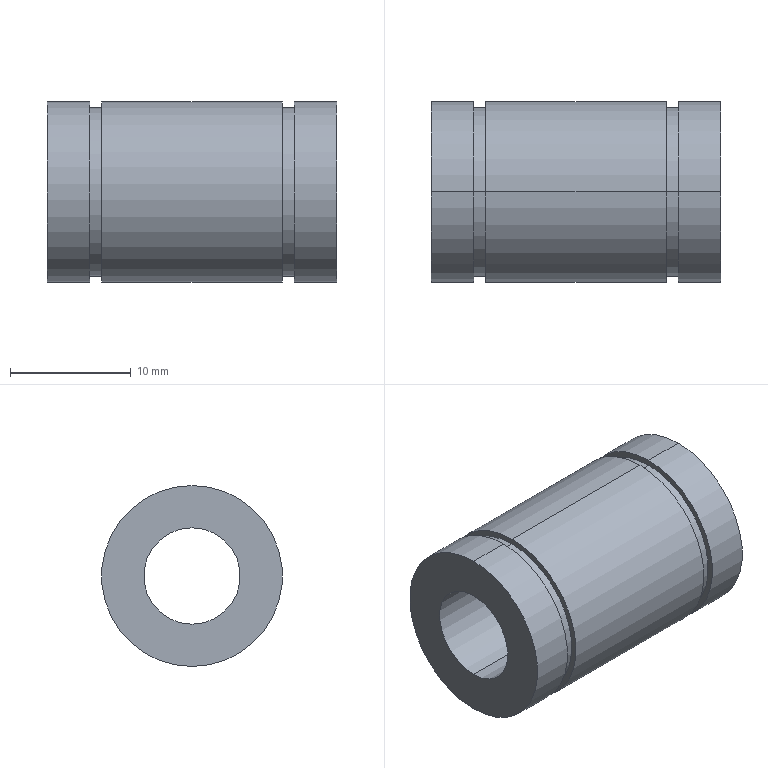Part | STEP file | linear bearing LM8-8-15-24 | 1 solid | 18 faces | box 24 x 15 x 15 mm | volume 2989 mm3 | cylinder 12 | plane 6 | commonest cylinder face diameters 15 x6 14 x4 8 x2
STEP:
#1=CARTESIAN_POINT('',(0.,0.,0.));
#2=DIRECTION('',(0.,0.,1.));
#3=DIRECTION('',(1.,0.,0.));
#4=AXIS2_PLACEMENT_3D('',#1,#2,#3);
#5=CARTESIAN_POINT('',(-20.214,0.,4.));
#6=VERTEX_POINT('',#5);
#7=CARTESIAN_POINT('',(-44.214,0.,4.));
#8=VERTEX_POINT('',#7);
#9=CARTESIAN_POINT('',(-96.213,0.,4.));
#10=DIRECTION('',(-1.,0.,0.));
#11=VECTOR('',#10,1.);
#12=LINE('',#9,#11);
#13=CARTESIAN_POINT('',(-96.213,0.,0.));
#14=DIRECTION('',(-1.,0.,0.));
#15=DIRECTION('',(0.,0.,1.));
#16=AXIS2_PLACEMENT_3D('',#13,#14,#15);
#17=CYLINDRICAL_SURFACE('',#16,4.);
#18=CARTESIAN_POINT('',(6.283,0.));
#19=DIRECTION('',(0.,1.));
#20=VECTOR('',#19,1.);
#21=LINE('',#18,#20);
#22=(GEOMETRIC_REPRESENTATION_CONTEXT(2)PARAMETRIC_REPRESENTATION_CONTEXT()REPRESENTATION_CONTEXT('',''));
#23=DEFINITIONAL_REPRESENTATION('',(#21),#22);
#24=PCURVE('',#17,#23);
#25=CARTESIAN_POINT('',(-96.213,0.,0.));
#26=DIRECTION('',(-1.,0.,0.));
#27=DIRECTION('',(0.,0.,1.));
#28=AXIS2_PLACEMENT_3D('',#25,#26,#27);
#29=CYLINDRICAL_SURFACE('',#28,4.);
#30=CARTESIAN_POINT('',(0.,0.));
#31=DIRECTION('',(0.,1.));
#32=VECTOR('',#31,1.);
#33=LINE('',#30,#32);
#34=(GEOMETRIC_REPRESENTATION_CONTEXT(2)PARAMETRIC_REPRESENTATION_CONTEXT()REPRESENTATION_CONTEXT('',''));
#35=DEFINITIONAL_REPRESENTATION('',(#33),#34);
#36=PCURVE('',#29,#35);
#37=SURFACE_CURVE('',#12,(#24,#36),.PCURVE_S1.);
#38=EDGE_CURVE('',#6,#8,#37,.T.);
#39=ORIENTED_EDGE('',*,*,#38,.T.);
#40=CARTESIAN_POINT('',(-44.214,0.,-4.));
#41=VERTEX_POINT('',#40);
#42=CARTESIAN_POINT('',(-44.214,0.,0.));
#43=DIRECTION('',(-1.,0.,0.));
#44=DIRECTION('',(0.,0.,1.));
#45=AXIS2_PLACEMENT_3D('',#42,#43,#44);
#46=CIRCLE('',#45,4.);
#47=CARTESIAN_POINT('',(0.,-51.999));
#48=DIRECTION('',(1.,0.));
#49=VECTOR('',#48,1.);
#50=LINE('',#47,#49);
#51=(GEOMETRIC_REPRESENTATION_CONTEXT(2)PARAMETRIC_REPRESENTATION_CONTEXT()REPRESENTATION_CONTEXT('',''));
#52=DEFINITIONAL_REPRESENTATION('',(#50),#51);
#53=PCURVE('',#17,#52);
#54=CARTESIAN_POINT('',(-44.214,4.,0.));
#55=DIRECTION('',(1.,0.,0.));
#56=DIRECTION('',(0.,0.,-1.));
#57=AXIS2_PLACEMENT_3D('',#54,#55,#56);
#58=PLANE('',#57);
#59=CARTESIAN_POINT('',(-4.,-4.));
#60=CARTESIAN_POINT('',(-4.,2.928));
#61=CARTESIAN_POINT('',(2.,-0.5359));
#62=CARTESIAN_POINT('',(8.,-4.));
#63=CARTESIAN_POINT('',(2.,-7.464));
#64=CARTESIAN_POINT('',(-4.,-10.928));
#65=CARTESIAN_POINT('',(-4.,-4.));
#66=(BOUNDED_CURVE()B_SPLINE_CURVE(2,(#59,#60,#61,#62,#63,#64,#65),.UNSPECIFIED.,.T.,.F.)B_SPLINE_CURVE_WITH_KNOTS((1,2,2,2,2,1),(-2.094,0.,2.094,4.189,6.283,8.378),.UNSPECIFIED.)CURVE()GEOMETRIC_REPRESENTATION_ITEM()RATIONAL_B_SPLINE_CURVE((1.,0.5,1.,0.5,1.,0.5,1.))REPRESENTATION_ITEM(''));
#67=(GEOMETRIC_REPRESENTATION_CONTEXT(2)PARAMETRIC_REPRESENTATION_CONTEXT()REPRESENTATION_CONTEXT('',''));
#68=DEFINITIONAL_REPRESENTATION('',(#66),#67);
#69=PCURVE('',#58,#68);
#70=SURFACE_CURVE('',#46,(#53,#69),.PCURVE_S1.);
#71=EDGE_CURVE('',#41,#8,#70,.T.);
#72=ORIENTED_EDGE('',*,*,#71,.F.);
#73=CARTESIAN_POINT('',(-20.214,0.,-4.));
#74=VERTEX_POINT('',#73);
#75=CARTESIAN_POINT('',(-96.213,0.,-4.));
#76=DIRECTION('',(-1.,0.,0.));
#77=VECTOR('',#76,1.);
#78=LINE('',#75,#77);
#79=CARTESIAN_POINT('',(3.142,0.));
#80=DIRECTION('',(0.,1.));
#81=VECTOR('',#80,1.);
#82=LINE('',#79,#81);
#83=(GEOMETRIC_REPRESENTATION_CONTEXT(2)PARAMETRIC_REPRESENTATION_CONTEXT()REPRESENTATION_CONTEXT('',''));
#84=DEFINITIONAL_REPRESENTATION('',(#82),#83);
#85=PCURVE('',#17,#84);
#86=CARTESIAN_POINT('',(3.142,0.));
#87=DIRECTION('',(0.,1.));
#88=VECTOR('',#87,1.);
#89=LINE('',#86,#88);
#90=(GEOMETRIC_REPRESENTATION_CONTEXT(2)PARAMETRIC_REPRESENTATION_CONTEXT()REPRESENTATION_CONTEXT('',''));
#91=DEFINITIONAL_REPRESENTATION('',(#89),#90);
#92=PCURVE('',#29,#91);
#93=SURFACE_CURVE('',#78,(#85,#92),.PCURVE_S1.);
#94=EDGE_CURVE('',#74,#41,#93,.T.);
#95=ORIENTED_EDGE('',*,*,#94,.F.);
#96=CARTESIAN_POINT('',(-20.214,0.,0.));
#97=DIRECTION('',(-1.,0.,0.));
#98=DIRECTION('',(0.,0.,1.));
#99=AXIS2_PLACEMENT_3D('',#96,#97,#98);
#100=CIRCLE('',#99,4.);
#101=CARTESIAN_POINT('',(0.,-75.999));
#102=DIRECTION('',(1.,0.));
#103=VECTOR('',#102,1.);
#104=LINE('',#101,#103);
#105=(GEOMETRIC_REPRESENTATION_CONTEXT(2)PARAMETRIC_REPRESENTATION_CONTEXT()REPRESENTATION_CONTEXT('',''));
#106=DEFINITIONAL_REPRESENTATION('',(#104),#105);
#107=PCURVE('',#17,#106);
#108=CARTESIAN_POINT('',(-20.214,4.,0.));
#109=DIRECTION('',(-1.,0.,0.));
#110=DIRECTION('',(0.,0.,1.));
#111=AXIS2_PLACEMENT_3D('',#108,#109,#110);
#112=PLANE('',#111);
#113=CARTESIAN_POINT('',(0.,-4.));
#114=DIRECTION('',(1.,0.));
#115=AXIS2_PLACEMENT_2D('',#113,#114);
#116=CIRCLE('',#115,4.);
#117=(GEOMETRIC_REPRESENTATION_CONTEXT(2)PARAMETRIC_REPRESENTATION_CONTEXT()REPRESENTATION_CONTEXT('',''));
#118=DEFINITIONAL_REPRESENTATION('',(#116),#117);
#119=PCURVE('',#112,#118);
#120=SURFACE_CURVE('',#100,(#107,#119),.PCURVE_S1.);
#121=EDGE_CURVE('',#74,#6,#120,.T.);
#122=ORIENTED_EDGE('',*,*,#121,.T.);
#123=EDGE_LOOP('',(#39,#72,#95,#122));
#124=FACE_BOUND('',#123,.F.);
#125=ADVANCED_FACE('',(#124),#17,.F.);
#126=CARTESIAN_POINT('',(-20.214,0.,7.5));
#127=VERTEX_POINT('',#126);
#128=CARTESIAN_POINT('',(-20.214,0.,-7.5));
#129=VERTEX_POINT('',#128);
#130=CARTESIAN_POINT('',(-20.214,0.,0.));
#131=DIRECTION('',(-1.,0.,0.));
#132=DIRECTION('',(0.,0.,1.));
#133=AXIS2_PLACEMENT_3D('',#130,#131,#132);
#134=CIRCLE('',#133,7.5);
#135=CARTESIAN_POINT('',(-96.213,0.,0.));
#136=DIRECTION('',(-1.,0.,0.));
#137=DIRECTION('',(0.,0.,1.));
#138=AXIS2_PLACEMENT_3D('',#135,#136,#137);
#139=CYLINDRICAL_SURFACE('',#138,7.5);
#140=CARTESIAN_POINT('',(0.,-75.999));
#141=DIRECTION('',(1.,0.));
#142=VECTOR('',#141,1.);
#143=LINE('',#140,#142);
#144=(GEOMETRIC_REPRESENTATION_CONTEXT(2)PARAMETRIC_REPRESENTATION_CONTEXT()REPRESENTATION_CONTEXT('',''));
#145=DEFINITIONAL_REPRESENTATION('',(#143),#144);
#146=PCURVE('',#139,#145);
#147=CARTESIAN_POINT('',(0.,-4.));
#148=DIRECTION('',(1.,0.));
#149=AXIS2_PLACEMENT_2D('',#147,#148);
#150=CIRCLE('',#149,7.5);
#151=(GEOMETRIC_REPRESENTATION_CONTEXT(2)PARAMETRIC_REPRESENTATION_CONTEXT()REPRESENTATION_CONTEXT('',''));
#152=DEFINITIONAL_REPRESENTATION('',(#150),#151);
#153=PCURVE('',#112,#152);
#154=SURFACE_CURVE('',#134,(#146,#153),.PCURVE_S1.);
#155=EDGE_CURVE('',#127,#129,#154,.T.);
#156=ORIENTED_EDGE('',*,*,#155,.T.);
#157=CARTESIAN_POINT('',(-23.714,0.,-7.5));
#158=VERTEX_POINT('',#157);
#159=CARTESIAN_POINT('',(-96.213,0.,-7.5));
#160=DIRECTION('',(-1.,0.,0.));
#161=VECTOR('',#160,1.);
#162=LINE('',#159,#161);
#163=CARTESIAN_POINT('',(3.142,0.));
#164=DIRECTION('',(0.,1.));
#165=VECTOR('',#164,1.);
#166=LINE('',#163,#165);
#167=(GEOMETRIC_REPRESENTATION_CONTEXT(2)PARAMETRIC_REPRESENTATION_CONTEXT()REPRESENTATION_CONTEXT('',''));
#168=DEFINITIONAL_REPRESENTATION('',(#166),#167);
#169=PCURVE('',#139,#168);
#170=CARTESIAN_POINT('',(-96.213,0.,0.));
#171=DIRECTION('',(-1.,0.,0.));
#172=DIRECTION('',(0.,0.,1.));
#173=AXIS2_PLACEMENT_3D('',#170,#171,#172);
#174=CYLINDRICAL_SURFACE('',#173,7.5);
#175=CARTESIAN_POINT('',(3.142,0.));
#176=DIRECTION('',(0.,1.));
#177=VECTOR('',#176,1.);
#178=LINE('',#175,#177);
#179=(GEOMETRIC_REPRESENTATION_CONTEXT(2)PARAMETRIC_REPRESENTATION_CONTEXT()REPRESENTATION_CONTEXT('',''));
#180=DEFINITIONAL_REPRESENTATION('',(#178),#179);
#181=PCURVE('',#174,#180);
#182=SURFACE_CURVE('',#162,(#169,#181),.PCURVE_S1.);
#183=EDGE_CURVE('',#129,#158,#182,.T.);
#184=ORIENTED_EDGE('',*,*,#183,.T.);
#185=CARTESIAN_POINT('',(-23.714,0.,7.5));
#186=VERTEX_POINT('',#185);
#187=CARTESIAN_POINT('',(-23.714,0.,0.));
#188=DIRECTION('',(-1.,0.,0.));
#189=DIRECTION('',(0.,0.,1.));
#190=AXIS2_PLACEMENT_3D('',#187,#188,#189);
#191=CIRCLE('',#190,7.5);
#192=CARTESIAN_POINT('',(0.,-72.499));
#193=DIRECTION('',(1.,0.));
#194=VECTOR('',#193,1.);
#195=LINE('',#192,#194);
#196=(GEOMETRIC_REPRESENTATION_CONTEXT(2)PARAMETRIC_REPRESENTATION_CONTEXT()REPRESENTATION_CONTEXT('',''));
#197=DEFINITIONAL_REPRESENTATION('',(#195),#196);
#198=PCURVE('',#139,#197);
#199=CARTESIAN_POINT('',(-23.714,7.5,0.));
#200=DIRECTION('',(1.,0.,0.));
#201=DIRECTION('',(0.,0.,-1.));
#202=AXIS2_PLACEMENT_3D('',#199,#200,#201);
#203=PLANE('',#202);
#204=CARTESIAN_POINT('',(-7.5,-7.5));
#205=CARTESIAN_POINT('',(-7.5,5.49));
#206=CARTESIAN_POINT('',(3.75,-1.005));
#207=CARTESIAN_POINT('',(15.,-7.5));
#208=CARTESIAN_POINT('',(3.75,-13.995));
#209=CARTESIAN_POINT('',(-7.5,-20.49));
#210=CARTESIAN_POINT('',(-7.5,-7.5));
#211=(BOUNDED_CURVE()B_SPLINE_CURVE(2,(#204,#205,#206,#207,#208,#209,#210),.UNSPECIFIED.,.T.,.F.)B_SPLINE_CURVE_WITH_KNOTS((1,2,2,2,2,1),(-2.094,0.,2.094,4.189,6.283,8.378),.UNSPECIFIED.)CURVE()GEOMETRIC_REPRESENTATION_ITEM()RATIONAL_B_SPLINE_CURVE((1.,0.5,1.,0.5,1.,0.5,1.))REPRESENTATION_ITEM(''));
#212=(GEOMETRIC_REPRESENTATION_CONTEXT(2)PARAMETRIC_REPRESENTATION_CONTEXT()REPRESENTATION_CONTEXT('',''));
#213=DEFINITIONAL_REPRESENTATION('',(#211),#212);
#214=PCURVE('',#203,#213);
#215=SURFACE_CURVE('',#191,(#198,#214),.PCURVE_S1.);
#216=EDGE_CURVE('',#186,#158,#215,.T.);
#217=ORIENTED_EDGE('',*,*,#216,.F.);
#218=CARTESIAN_POINT('',(-96.213,0.,7.5));
#219=DIRECTION('',(-1.,0.,0.));
#220=VECTOR('',#219,1.);
#221=LINE('',#218,#220);
#222=CARTESIAN_POINT('',(0.,0.));
#223=DIRECTION('',(0.,1.));
#224=VECTOR('',#223,1.);
#225=LINE('',#222,#224);
#226=(GEOMETRIC_REPRESENTATION_CONTEXT(2)PARAMETRIC_REPRESENTATION_CONTEXT()REPRESENTATION_CONTEXT('',''));
#227=DEFINITIONAL_REPRESENTATION('',(#225),#226);
#228=PCURVE('',#139,#227);
#229=CARTESIAN_POINT('',(6.283,0.));
#230=DIRECTION('',(0.,1.));
#231=VECTOR('',#230,1.);
#232=LINE('',#229,#231);
#233=(GEOMETRIC_REPRESENTATION_CONTEXT(2)PARAMETRIC_REPRESENTATION_CONTEXT()REPRESENTATION_CONTEXT('',''));
#234=DEFINITIONAL_REPRESENTATION('',(#232),#233);
#235=PCURVE('',#174,#234);
#236=SURFACE_CURVE('',#221,(#228,#235),.PCURVE_S1.);
#237=EDGE_CURVE('',#127,#186,#236,.T.);
#238=ORIENTED_EDGE('',*,*,#237,.F.);
#239=EDGE_LOOP('',(#156,#184,#217,#238));
#240=FACE_BOUND('',#239,.T.);
#241=ADVANCED_FACE('',(#240),#139,.T.);
#242=CARTESIAN_POINT('',(-23.714,0.,7.));
#243=VERTEX_POINT('',#242);
#244=CARTESIAN_POINT('',(-23.714,0.,-7.));
#245=VERTEX_POINT('',#244);
#246=CARTESIAN_POINT('',(-23.714,0.,0.));
#247=DIRECTION('',(-1.,0.,0.));
#248=DIRECTION('',(0.,0.,1.));
#249=AXIS2_PLACEMENT_3D('',#246,#247,#248);
#250=CIRCLE('',#249,7.);
#251=CARTESIAN_POINT('',(-96.213,0.,0.));
#252=DIRECTION('',(-1.,0.,0.));
#253=DIRECTION('',(0.,0.,1.));
#254=AXIS2_PLACEMENT_3D('',#251,#252,#253);
#255=CYLINDRICAL_SURFACE('',#254,7.);
#256=CARTESIAN_POINT('',(0.,-72.499));
#257=DIRECTION('',(1.,0.));
#258=VECTOR('',#257,1.);
#259=LINE('',#256,#258);
#260=(GEOMETRIC_REPRESENTATION_CONTEXT(2)PARAMETRIC_REPRESENTATION_CONTEXT()REPRESENTATION_CONTEXT('',''));
#261=DEFINITIONAL_REPRESENTATION('',(#259),#260);
#262=PCURVE('',#255,#261);
#263=CARTESIAN_POINT('',(-7.,-7.5));
#264=CARTESIAN_POINT('',(-7.,4.624));
#265=CARTESIAN_POINT('',(3.5,-1.438));
#266=CARTESIAN_POINT('',(14.,-7.5));
#267=CARTESIAN_POINT('',(3.5,-13.562));
#268=CARTESIAN_POINT('',(-7.,-19.624));
#269=CARTESIAN_POINT('',(-7.,-7.5));
#270=(BOUNDED_CURVE()B_SPLINE_CURVE(2,(#263,#264,#265,#266,#267,#268,#269),.UNSPECIFIED.,.T.,.F.)B_SPLINE_CURVE_WITH_KNOTS((1,2,2,2,2,1),(-2.094,0.,2.094,4.189,6.283,8.378),.UNSPECIFIED.)CURVE()GEOMETRIC_REPRESENTATION_ITEM()RATIONAL_B_SPLINE_CURVE((1.,0.5,1.,0.5,1.,0.5,1.))REPRESENTATION_ITEM(''));
#271=(GEOMETRIC_REPRESENTATION_CONTEXT(2)PARAMETRIC_REPRESENTATION_CONTEXT()REPRESENTATION_CONTEXT('',''));
#272=DEFINITIONAL_REPRESENTATION('',(#270),#271);
#273=PCURVE('',#203,#272);
#274=SURFACE_CURVE('',#250,(#262,#273),.PCURVE_S1.);
#275=EDGE_CURVE('',#243,#245,#274,.T.);
#276=ORIENTED_EDGE('',*,*,#275,.T.);
#277=CARTESIAN_POINT('',(-24.714,0.,-7.));
#278=VERTEX_POINT('',#277);
#279=CARTESIAN_POINT('',(-96.213,0.,-7.));
#280=DIRECTION('',(-1.,0.,0.));
#281=VECTOR('',#280,1.);
#282=LINE('',#279,#281);
#283=CARTESIAN_POINT('',(3.142,0.));
#284=DIRECTION('',(0.,1.));
#285=VECTOR('',#284,1.);
#286=LINE('',#283,#285);
#287=(GEOMETRIC_REPRESENTATION_CONTEXT(2)PARAMETRIC_REPRESENTATION_CONTEXT()REPRESENTATION_CONTEXT('',''));
#288=DEFINITIONAL_REPRESENTATION('',(#286),#287);
#289=PCURVE('',#255,#288);
#290=CARTESIAN_POINT('',(-96.213,0.,0.));
#291=DIRECTION('',(-1.,0.,0.));
#292=DIRECTION('',(0.,0.,1.));
#293=AXIS2_PLACEMENT_3D('',#290,#291,#292);
#294=CYLINDRICAL_SURFACE('',#293,7.);
#295=CARTESIAN_POINT('',(3.142,0.));
#296=DIRECTION('',(0.,1.));
#297=VECTOR('',#296,1.);
#298=LINE('',#295,#297);
#299=(GEOMETRIC_REPRESENTATION_CONTEXT(2)PARAMETRIC_REPRESENTATION_CONTEXT()REPRESENTATION_CONTEXT('',''));
#300=DEFINITIONAL_REPRESENTATION('',(#298),#299);
#301=PCURVE('',#294,#300);
#302=SURFACE_CURVE('',#282,(#289,#301),.PCURVE_S1.);
#303=EDGE_CURVE('',#245,#278,#302,.T.);
#304=ORIENTED_EDGE('',*,*,#303,.T.);
#305=CARTESIAN_POINT('',(-24.714,0.,7.));
#306=VERTEX_POINT('',#305);
#307=CARTESIAN_POINT('',(-24.714,0.,0.));
#308=DIRECTION('',(-1.,0.,0.));
#309=DIRECTION('',(0.,0.,1.));
#310=AXIS2_PLACEMENT_3D('',#307,#308,#309);
#311=CIRCLE('',#310,7.);
#312=CARTESIAN_POINT('',(0.,-71.499));
#313=DIRECTION('',(1.,0.));
#314=VECTOR('',#313,1.);
#315=LINE('',#312,#314);
#316=(GEOMETRIC_REPRESENTATION_CONTEXT(2)PARAMETRIC_REPRESENTATION_CONTEXT()REPRESENTATION_CONTEXT('',''));
#317=DEFINITIONAL_REPRESENTATION('',(#315),#316);
#318=PCURVE('',#255,#317);
#319=CARTESIAN_POINT('',(-24.714,7.5,0.));
#320=DIRECTION('',(-1.,0.,0.));
#321=DIRECTION('',(0.,0.,1.));
#322=AXIS2_PLACEMENT_3D('',#319,#320,#321);
#323=PLANE('',#322);
#324=CARTESIAN_POINT('',(0.,-7.5));
#325=DIRECTION('',(1.,0.));
#326=AXIS2_PLACEMENT_2D('',#324,#325);
#327=CIRCLE('',#326,7.);
#328=(GEOMETRIC_REPRESENTATION_CONTEXT(2)PARAMETRIC_REPRESENTATION_CONTEXT()REPRESENTATION_CONTEXT('',''));
#329=DEFINITIONAL_REPRESENTATION('',(#327),#328);
#330=PCURVE('',#323,#329);
#331=SURFACE_CURVE('',#311,(#318,#330),.PCURVE_S1.);
#332=EDGE_CURVE('',#306,#278,#331,.T.);
#333=ORIENTED_EDGE('',*,*,#332,.F.);
#334=CARTESIAN_POINT('',(-96.213,0.,7.));
#335=DIRECTION('',(-1.,0.,0.));
#336=VECTOR('',#335,1.);
#337=LINE('',#334,#336);
#338=CARTESIAN_POINT('',(0.,0.));
#339=DIRECTION('',(0.,1.));
#340=VECTOR('',#339,1.);
#341=LINE('',#338,#340);
#342=(GEOMETRIC_REPRESENTATION_CONTEXT(2)PARAMETRIC_REPRESENTATION_CONTEXT()REPRESENTATION_CONTEXT('',''));
#343=DEFINITIONAL_REPRESENTATION('',(#341),#342);
#344=PCURVE('',#255,#343);
#345=CARTESIAN_POINT('',(6.283,0.));
#346=DIRECTION('',(0.,1.));
#347=VECTOR('',#346,1.);
#348=LINE('',#345,#347);
#349=(GEOMETRIC_REPRESENTATION_CONTEXT(2)PARAMETRIC_REPRESENTATION_CONTEXT()REPRESENTATION_CONTEXT('',''));
#350=DEFINITIONAL_REPRESENTATION('',(#348),#349);
#351=PCURVE('',#294,#350);
#352=SURFACE_CURVE('',#337,(#344,#351),.PCURVE_S1.);
#353=EDGE_CURVE('',#243,#306,#352,.T.);
#354=ORIENTED_EDGE('',*,*,#353,.F.);
#355=EDGE_LOOP('',(#276,#304,#333,#354));
#356=FACE_BOUND('',#355,.T.);
#357=ADVANCED_FACE('',(#356),#255,.T.);
#358=CARTESIAN_POINT('',(-24.714,0.,7.5));
#359=VERTEX_POINT('',#358);
#360=CARTESIAN_POINT('',(-24.714,0.,-7.5));
#361=VERTEX_POINT('',#360);
#362=CARTESIAN_POINT('',(-24.714,0.,0.));
#363=DIRECTION('',(-1.,0.,0.));
#364=DIRECTION('',(0.,0.,1.));
#365=AXIS2_PLACEMENT_3D('',#362,#363,#364);
#366=CIRCLE('',#365,7.5);
#367=CARTESIAN_POINT('',(-96.213,0.,0.));
#368=DIRECTION('',(-1.,0.,0.));
#369=DIRECTION('',(0.,0.,1.));
#370=AXIS2_PLACEMENT_3D('',#367,#368,#369);
#371=CYLINDRICAL_SURFACE('',#370,7.5);
#372=CARTESIAN_POINT('',(0.,-71.499));
#373=DIRECTION('',(1.,0.));
#374=VECTOR('',#373,1.);
#375=LINE('',#372,#374);
#376=(GEOMETRIC_REPRESENTATION_CONTEXT(2)PARAMETRIC_REPRESENTATION_CONTEXT()REPRESENTATION_CONTEXT('',''));
#377=DEFINITIONAL_REPRESENTATION('',(#375),#376);
#378=PCURVE('',#371,#377);
#379=CARTESIAN_POINT('',(0.,-7.5));
#380=DIRECTION('',(1.,0.));
#381=AXIS2_PLACEMENT_2D('',#379,#380);
#382=CIRCLE('',#381,7.5);
#383=(GEOMETRIC_REPRESENTATION_CONTEXT(2)PARAMETRIC_REPRESENTATION_CONTEXT()REPRESENTATION_CONTEXT('',''));
#384=DEFINITIONAL_REPRESENTATION('',(#382),#383);
#385=PCURVE('',#323,#384);
#386=SURFACE_CURVE('',#366,(#378,#385),.PCURVE_S1.);
#387=EDGE_CURVE('',#359,#361,#386,.T.);
#388=ORIENTED_EDGE('',*,*,#387,.T.);
#389=CARTESIAN_POINT('',(-39.714,0.,-7.5));
#390=VERTEX_POINT('',#389);
#391=CARTESIAN_POINT('',(-96.213,0.,-7.5));
#392=DIRECTION('',(-1.,0.,0.));
#393=VECTOR('',#392,1.);
#394=LINE('',#391,#393);
#395=CARTESIAN_POINT('',(3.142,0.));
#396=DIRECTION('',(0.,1.));
#397=VECTOR('',#396,1.);
#398=LINE('',#395,#397);
#399=(GEOMETRIC_REPRESENTATION_CONTEXT(2)PARAMETRIC_REPRESENTATION_CONTEXT()REPRESENTATION_CONTEXT('',''));
#400=DEFINITIONAL_REPRESENTATION('',(#398),#399);
#401=PCURVE('',#371,#400);
#402=CARTESIAN_POINT('',(-96.213,0.,0.));
#403=DIRECTION('',(-1.,0.,0.));
#404=DIRECTION('',(0.,0.,1.));
#405=AXIS2_PLACEMENT_3D('',#402,#403,#404);
#406=CYLINDRICAL_SURFACE('',#405,7.5);
#407=CARTESIAN_POINT('',(3.142,0.));
#408=DIRECTION('',(0.,1.));
#409=VECTOR('',#408,1.);
#410=LINE('',#407,#409);
#411=(GEOMETRIC_REPRESENTATION_CONTEXT(2)PARAMETRIC_REPRESENTATION_CONTEXT()REPRESENTATION_CONTEXT('',''));
#412=DEFINITIONAL_REPRESENTATION('',(#410),#411);
#413=PCURVE('',#406,#412);
#414=SURFACE_CURVE('',#394,(#401,#413),.PCURVE_S1.);
#415=EDGE_CURVE('',#361,#390,#414,.T.);
#416=ORIENTED_EDGE('',*,*,#415,.T.);
#417=CARTESIAN_POINT('',(-39.714,0.,7.5));
#418=VERTEX_POINT('',#417);
#419=CARTESIAN_POINT('',(-39.714,0.,0.));
#420=DIRECTION('',(-1.,0.,0.));
#421=DIRECTION('',(0.,0.,1.));
#422=AXIS2_PLACEMENT_3D('',#419,#420,#421);
#423=CIRCLE('',#422,7.5);
#424=CARTESIAN_POINT('',(0.,-56.499));
#425=DIRECTION('',(1.,0.));
#426=VECTOR('',#425,1.);
#427=LINE('',#424,#426);
#428=(GEOMETRIC_REPRESENTATION_CONTEXT(2)PARAMETRIC_REPRESENTATION_CONTEXT()REPRESENTATION_CONTEXT('',''));
#429=DEFINITIONAL_REPRESENTATION('',(#427),#428);
#430=PCURVE('',#371,#429);
#431=CARTESIAN_POINT('',(-39.714,7.5,0.));
#432=DIRECTION('',(1.,0.,0.));
#433=DIRECTION('',(0.,0.,-1.));
#434=AXIS2_PLACEMENT_3D('',#431,#432,#433);
#435=PLANE('',#434);
#436=CARTESIAN_POINT('',(-7.5,-7.5));
#437=CARTESIAN_POINT('',(-7.5,5.49));
#438=CARTESIAN_POINT('',(3.75,-1.005));
#439=CARTESIAN_POINT('',(15.,-7.5));
#440=CARTESIAN_POINT('',(3.75,-13.995));
#441=CARTESIAN_POINT('',(-7.5,-20.49));
#442=CARTESIAN_POINT('',(-7.5,-7.5));
#443=(BOUNDED_CURVE()B_SPLINE_CURVE(2,(#436,#437,#438,#439,#440,#441,#442),.UNSPECIFIED.,.T.,.F.)B_SPLINE_CURVE_WITH_KNOTS((1,2,2,2,2,1),(-2.094,0.,2.094,4.189,6.283,8.378),.UNSPECIFIED.)CURVE()GEOMETRIC_REPRESENTATION_ITEM()RATIONAL_B_SPLINE_CURVE((1.,0.5,1.,0.5,1.,0.5,1.))REPRESENTATION_ITEM(''));
#444=(GEOMETRIC_REPRESENTATION_CONTEXT(2)PARAMETRIC_REPRESENTATION_CONTEXT()REPRESENTATION_CONTEXT('',''));
#445=DEFINITIONAL_REPRESENTATION('',(#443),#444);
#446=PCURVE('',#435,#445);
#447=SURFACE_CURVE('',#423,(#430,#446),.PCURVE_S1.);
#448=EDGE_CURVE('',#418,#390,#447,.T.);
#449=ORIENTED_EDGE('',*,*,#448,.F.);
#450=CARTESIAN_POINT('',(-96.213,0.,7.5));
#451=DIRECTION('',(-1.,0.,0.));
#452=VECTOR('',#451,1.);
#453=LINE('',#450,#452);
#454=CARTESIAN_POINT('',(0.,0.));
#455=DIRECTION('',(0.,1.));
#456=VECTOR('',#455,1.);
#457=LINE('',#454,#456);
#458=(GEOMETRIC_REPRESENTATION_CONTEXT(2)PARAMETRIC_REPRESENTATION_CONTEXT()REPRESENTATION_CONTEXT('',''));
#459=DEFINITIONAL_REPRESENTATION('',(#457),#458);
#460=PCURVE('',#371,#459);
#461=CARTESIAN_POINT('',(6.283,0.));
#462=DIRECTION('',(0.,1.));
#463=VECTOR('',#462,1.);
#464=LINE('',#461,#463);
#465=(GEOMETRIC_REPRESENTATION_CONTEXT(2)PARAMETRIC_REPRESENTATION_CONTEXT()REPRESENTATION_CONTEXT('',''));
#466=DEFINITIONAL_REPRESENTATION('',(#464),#465);
#467=PCURVE('',#406,#466);
#468=SURFACE_CURVE('',#453,(#460,#467),.PCURVE_S1.);
#469=EDGE_CURVE('',#359,#418,#468,.T.);
#470=ORIENTED_EDGE('',*,*,#469,.F.);
#471=EDGE_LOOP('',(#388,#416,#449,#470));
#472=FACE_BOUND('',#471,.T.);
#473=ADVANCED_FACE('',(#472),#371,.T.);
#474=CARTESIAN_POINT('',(-39.714,0.,7.));
#475=VERTEX_POINT('',#474);
#476=CARTESIAN_POINT('',(-39.714,0.,-7.));
#477=VERTEX_POINT('',#476);
#478=CARTESIAN_POINT('',(-39.714,0.,0.));
#479=DIRECTION('',(-1.,0.,0.));
#480=DIRECTION('',(0.,0.,1.));
#481=AXIS2_PLACEMENT_3D('',#478,#479,#480);
#482=CIRCLE('',#481,7.);
#483=CARTESIAN_POINT('',(-96.213,0.,0.));
#484=DIRECTION('',(-1.,0.,0.));
#485=DIRECTION('',(0.,0.,1.));
#486=AXIS2_PLACEMENT_3D('',#483,#484,#485);
#487=CYLINDRICAL_SURFACE('',#486,7.);
#488=CARTESIAN_POINT('',(0.,-56.499));
#489=DIRECTION('',(1.,0.));
#490=VECTOR('',#489,1.);
#491=LINE('',#488,#490);
#492=(GEOMETRIC_REPRESENTATION_CONTEXT(2)PARAMETRIC_REPRESENTATION_CONTEXT()REPRESENTATION_CONTEXT('',''));
#493=DEFINITIONAL_REPRESENTATION('',(#491),#492);
#494=PCURVE('',#487,#493);
#495=CARTESIAN_POINT('',(-7.,-7.5));
#496=CARTESIAN_POINT('',(-7.,4.624));
#497=CARTESIAN_POINT('',(3.5,-1.438));
#498=CARTESIAN_POINT('',(14.,-7.5));
#499=CARTESIAN_POINT('',(3.5,-13.562));
#500=CARTESIAN_POINT('',(-7.,-19.624));
#501=CARTESIAN_POINT('',(-7.,-7.5));
#502=(BOUNDED_CURVE()B_SPLINE_CURVE(2,(#495,#496,#497,#498,#499,#500,#501),.UNSPECIFIED.,.T.,.F.)B_SPLINE_CURVE_WITH_KNOTS((1,2,2,2,2,1),(-2.094,0.,2.094,4.189,6.283,8.378),.UNSPECIFIED.)CURVE()GEOMETRIC_REPRESENTATION_ITEM()RATIONAL_B_SPLINE_CURVE((1.,0.5,1.,0.5,1.,0.5,1.))REPRESENTATION_ITEM(''));
#503=(GEOMETRIC_REPRESENTATION_CONTEXT(2)PARAMETRIC_REPRESENTATION_CONTEXT()REPRESENTATION_CONTEXT('',''));
#504=DEFINITIONAL_REPRESENTATION('',(#502),#503);
#505=PCURVE('',#435,#504);
#506=SURFACE_CURVE('',#482,(#494,#505),.PCURVE_S1.);
#507=EDGE_CURVE('',#475,#477,#506,.T.);
#508=ORIENTED_EDGE('',*,*,#507,.T.);
#509=CARTESIAN_POINT('',(-40.714,0.,-7.));
#510=VERTEX_POINT('',#509);
#511=CARTESIAN_POINT('',(-96.213,0.,-7.));
#512=DIRECTION('',(-1.,0.,0.));
#513=VECTOR('',#512,1.);
#514=LINE('',#511,#513);
#515=CARTESIAN_POINT('',(3.142,0.));
#516=DIRECTION('',(0.,1.));
#517=VECTOR('',#516,1.);
#518=LINE('',#515,#517);
#519=(GEOMETRIC_REPRESENTATION_CONTEXT(2)PARAMETRIC_REPRESENTATION_CONTEXT()REPRESENTATION_CONTEXT('',''));
#520=DEFINITIONAL_REPRESENTATION('',(#518),#519);
#521=PCURVE('',#487,#520);
#522=CARTESIAN_POINT('',(-96.213,0.,0.));
#523=DIRECTION('',(-1.,0.,0.));
#524=DIRECTION('',(0.,0.,1.));
#525=AXIS2_PLACEMENT_3D('',#522,#523,#524);
#526=CYLINDRICAL_SURFACE('',#525,7.);
#527=CARTESIAN_POINT('',(3.142,0.));
#528=DIRECTION('',(0.,1.));
#529=VECTOR('',#528,1.);
#530=LINE('',#527,#529);
#531=(GEOMETRIC_REPRESENTATION_CONTEXT(2)PARAMETRIC_REPRESENTATION_CONTEXT()REPRESENTATION_CONTEXT('',''));
#532=DEFINITIONAL_REPRESENTATION('',(#530),#531);
#533=PCURVE('',#526,#532);
#534=SURFACE_CURVE('',#514,(#521,#533),.PCURVE_S1.);
#535=EDGE_CURVE('',#477,#510,#534,.T.);
#536=ORIENTED_EDGE('',*,*,#535,.T.);
#537=CARTESIAN_POINT('',(-40.714,0.,7.));
#538=VERTEX_POINT('',#537);
#539=CARTESIAN_POINT('',(-40.714,0.,0.));
#540=DIRECTION('',(-1.,0.,0.));
#541=DIRECTION('',(0.,0.,1.));
#542=AXIS2_PLACEMENT_3D('',#539,#540,#541);
#543=CIRCLE('',#542,7.);
#544=CARTESIAN_POINT('',(0.,-55.499));
#545=DIRECTION('',(1.,0.));
#546=VECTOR('',#545,1.);
#547=LINE('',#544,#546);
#548=(GEOMETRIC_REPRESENTATION_CONTEXT(2)PARAMETRIC_REPRESENTATION_CONTEXT()REPRESENTATION_CONTEXT('',''));
#549=DEFINITIONAL_REPRESENTATION('',(#547),#548);
#550=PCURVE('',#487,#549);
#551=CARTESIAN_POINT('',(-40.714,7.5,0.));
#552=DIRECTION('',(-1.,0.,0.));
#553=DIRECTION('',(0.,0.,1.));
#554=AXIS2_PLACEMENT_3D('',#551,#552,#553);
#555=PLANE('',#554);
#556=CARTESIAN_POINT('',(0.,-7.5));
#557=DIRECTION('',(1.,0.));
#558=AXIS2_PLACEMENT_2D('',#556,#557);
#559=CIRCLE('',#558,7.);
#560=(GEOMETRIC_REPRESENTATION_CONTEXT(2)PARAMETRIC_REPRESENTATION_CONTEXT()REPRESENTATION_CONTEXT('',''));
#561=DEFINITIONAL_REPRESENTATION('',(#559),#560);
#562=PCURVE('',#555,#561);
#563=SURFACE_CURVE('',#543,(#550,#562),.PCURVE_S1.);
#564=EDGE_CURVE('',#538,#510,#563,.T.);
#565=ORIENTED_EDGE('',*,*,#564,.F.);
#566=CARTESIAN_POINT('',(-96.213,0.,7.));
#567=DIRECTION('',(-1.,0.,0.));
#568=VECTOR('',#567,1.);
#569=LINE('',#566,#568);
#570=CARTESIAN_POINT('',(0.,0.));
#571=DIRECTION('',(0.,1.));
#572=VECTOR('',#571,1.);
#573=LINE('',#570,#572);
#574=(GEOMETRIC_REPRESENTATION_CONTEXT(2)PARAMETRIC_REPRESENTATION_CONTEXT()REPRESENTATION_CONTEXT('',''));
#575=DEFINITIONAL_REPRESENTATION('',(#573),#574);
#576=PCURVE('',#487,#575);
#577=CARTESIAN_POINT('',(6.283,0.));
#578=DIRECTION('',(0.,1.));
#579=VECTOR('',#578,1.);
#580=LINE('',#577,#579);
#581=(GEOMETRIC_REPRESENTATION_CONTEXT(2)PARAMETRIC_REPRESENTATION_CONTEXT()REPRESENTATION_CONTEXT('',''));
#582=DEFINITIONAL_REPRESENTATION('',(#580),#581);
#583=PCURVE('',#526,#582);
#584=SURFACE_CURVE('',#569,(#576,#583),.PCURVE_S1.);
#585=EDGE_CURVE('',#475,#538,#584,.T.);
#586=ORIENTED_EDGE('',*,*,#585,.F.);
#587=EDGE_LOOP('',(#508,#536,#565,#586));
#588=FACE_BOUND('',#587,.T.);
#589=ADVANCED_FACE('',(#588),#487,.T.);
#590=CARTESIAN_POINT('',(-40.714,0.,7.5));
#591=VERTEX_POINT('',#590);
#592=CARTESIAN_POINT('',(-40.714,0.,-7.5));
#593=VERTEX_POINT('',#592);
#594=CARTESIAN_POINT('',(-40.714,0.,0.));
#595=DIRECTION('',(-1.,0.,0.));
#596=DIRECTION('',(0.,0.,1.));
#597=AXIS2_PLACEMENT_3D('',#594,#595,#596);
#598=CIRCLE('',#597,7.5);
#599=CARTESIAN_POINT('',(-96.213,0.,0.));
#600=DIRECTION('',(-1.,0.,0.));
#601=DIRECTION('',(0.,0.,1.));
#602=AXIS2_PLACEMENT_3D('',#599,#600,#601);
#603=CYLINDRICAL_SURFACE('',#602,7.5);
#604=CARTESIAN_POINT('',(0.,-55.499));
#605=DIRECTION('',(1.,0.));
#606=VECTOR('',#605,1.);
#607=LINE('',#604,#606);
#608=(GEOMETRIC_REPRESENTATION_CONTEXT(2)PARAMETRIC_REPRESENTATION_CONTEXT()REPRESENTATION_CONTEXT('',''));
#609=DEFINITIONAL_REPRESENTATION('',(#607),#608);
#610=PCURVE('',#603,#609);
#611=CARTESIAN_POINT('',(0.,-7.5));
#612=DIRECTION('',(1.,0.));
#613=AXIS2_PLACEMENT_2D('',#611,#612);
#614=CIRCLE('',#613,7.5);
#615=(GEOMETRIC_REPRESENTATION_CONTEXT(2)PARAMETRIC_REPRESENTATION_CONTEXT()REPRESENTATION_CONTEXT('',''));
#616=DEFINITIONAL_REPRESENTATION('',(#614),#615);
#617=PCURVE('',#555,#616);
#618=SURFACE_CURVE('',#598,(#610,#617),.PCURVE_S1.);
#619=EDGE_CURVE('',#591,#593,#618,.T.);
#620=ORIENTED_EDGE('',*,*,#619,.T.);
#621=CARTESIAN_POINT('',(-44.214,0.,-7.5));
#622=VERTEX_POINT('',#621);
#623=CARTESIAN_POINT('',(-96.213,0.,-7.5));
#624=DIRECTION('',(-1.,0.,0.));
#625=VECTOR('',#624,1.);
#626=LINE('',#623,#625);
#627=CARTESIAN_POINT('',(3.142,0.));
#628=DIRECTION('',(0.,1.));
#629=VECTOR('',#628,1.);
#630=LINE('',#627,#629);
#631=(GEOMETRIC_REPRESENTATION_CONTEXT(2)PARAMETRIC_REPRESENTATION_CONTEXT()REPRESENTATION_CONTEXT('',''));
#632=DEFINITIONAL_REPRESENTATION('',(#630),#631);
#633=PCURVE('',#603,#632);
#634=CARTESIAN_POINT('',(-96.213,0.,0.));
#635=DIRECTION('',(-1.,0.,0.));
#636=DIRECTION('',(0.,0.,1.));
#637=AXIS2_PLACEMENT_3D('',#634,#635,#636);
#638=CYLINDRICAL_SURFACE('',#637,7.5);
#639=CARTESIAN_POINT('',(3.142,0.));
#640=DIRECTION('',(0.,1.));
#641=VECTOR('',#640,1.);
#642=LINE('',#639,#641);
#643=(GEOMETRIC_REPRESENTATION_CONTEXT(2)PARAMETRIC_REPRESENTATION_CONTEXT()REPRESENTATION_CONTEXT('',''));
#644=DEFINITIONAL_REPRESENTATION('',(#642),#643);
#645=PCURVE('',#638,#644);
#646=SURFACE_CURVE('',#626,(#633,#645),.PCURVE_S1.);
#647=EDGE_CURVE('',#593,#622,#646,.T.);
#648=ORIENTED_EDGE('',*,*,#647,.T.);
#649=CARTESIAN_POINT('',(-44.214,0.,7.5));
#650=VERTEX_POINT('',#649);
#651=CARTESIAN_POINT('',(-44.214,0.,0.));
#652=DIRECTION('',(-1.,0.,0.));
#653=DIRECTION('',(0.,0.,1.));
#654=AXIS2_PLACEMENT_3D('',#651,#652,#653);
#655=CIRCLE('',#654,7.5);
#656=CARTESIAN_POINT('',(0.,-51.999));
#657=DIRECTION('',(1.,0.));
#658=VECTOR('',#657,1.);
#659=LINE('',#656,#658);
#660=(GEOMETRIC_REPRESENTATION_CONTEXT(2)PARAMETRIC_REPRESENTATION_CONTEXT()REPRESENTATION_CONTEXT('',''));
#661=DEFINITIONAL_REPRESENTATION('',(#659),#660);
#662=PCURVE('',#603,#661);
#663=CARTESIAN_POINT('',(-7.5,-4.));
#664=CARTESIAN_POINT('',(-7.5,8.99));
#665=CARTESIAN_POINT('',(3.75,2.495));
#666=CARTESIAN_POINT('',(15.,-4.));
#667=CARTESIAN_POINT('',(3.75,-10.495));
#668=CARTESIAN_POINT('',(-7.5,-16.99));
#669=CARTESIAN_POINT('',(-7.5,-4.));
#670=(BOUNDED_CURVE()B_SPLINE_CURVE(2,(#663,#664,#665,#666,#667,#668,#669),.UNSPECIFIED.,.T.,.F.)B_SPLINE_CURVE_WITH_KNOTS((1,2,2,2,2,1),(-2.094,0.,2.094,4.189,6.283,8.378),.UNSPECIFIED.)CURVE()GEOMETRIC_REPRESENTATION_ITEM()RATIONAL_B_SPLINE_CURVE((1.,0.5,1.,0.5,1.,0.5,1.))REPRESENTATION_ITEM(''));
#671=(GEOMETRIC_REPRESENTATION_CONTEXT(2)PARAMETRIC_REPRESENTATION_CONTEXT()REPRESENTATION_CONTEXT('',''));
#672=DEFINITIONAL_REPRESENTATION('',(#670),#671);
#673=PCURVE('',#58,#672);
#674=SURFACE_CURVE('',#655,(#662,#673),.PCURVE_S1.);
#675=EDGE_CURVE('',#650,#622,#674,.T.);
#676=ORIENTED_EDGE('',*,*,#675,.F.);
#677=CARTESIAN_POINT('',(-96.213,0.,7.5));
#678=DIRECTION('',(-1.,0.,0.));
#679=VECTOR('',#678,1.);
#680=LINE('',#677,#679);
#681=CARTESIAN_POINT('',(0.,0.));
#682=DIRECTION('',(0.,1.));
#683=VECTOR('',#682,1.);
#684=LINE('',#681,#683);
#685=(GEOMETRIC_REPRESENTATION_CONTEXT(2)PARAMETRIC_REPRESENTATION_CONTEXT()REPRESENTATION_CONTEXT('',''));
#686=DEFINITIONAL_REPRESENTATION('',(#684),#685);
#687=PCURVE('',#603,#686);
#688=CARTESIAN_POINT('',(6.283,0.));
#689=DIRECTION('',(0.,1.));
#690=VECTOR('',#689,1.);
#691=LINE('',#688,#690);
#692=(GEOMETRIC_REPRESENTATION_CONTEXT(2)PARAMETRIC_REPRESENTATION_CONTEXT()REPRESENTATION_CONTEXT('',''));
#693=DEFINITIONAL_REPRESENTATION('',(#691),#692);
#694=PCURVE('',#638,#693);
#695=SURFACE_CURVE('',#680,(#687,#694),.PCURVE_S1.);
#696=EDGE_CURVE('',#591,#650,#695,.T.);
#697=ORIENTED_EDGE('',*,*,#696,.F.);
#698=EDGE_LOOP('',(#620,#648,#676,#697));
#699=FACE_BOUND('',#698,.T.);
#700=ADVANCED_FACE('',(#699),#603,.T.);
#701=CARTESIAN_POINT('',(-44.214,0.,0.));
#702=DIRECTION('',(-1.,0.,0.));
#703=DIRECTION('',(0.,0.,1.));
#704=AXIS2_PLACEMENT_3D('',#701,#702,#703);
#705=CIRCLE('',#704,4.);
#706=CARTESIAN_POINT('',(-4.,-4.));
#707=CARTESIAN_POINT('',(-4.,2.928));
#708=CARTESIAN_POINT('',(2.,-0.5359));
#709=CARTESIAN_POINT('',(8.,-4.));
#710=CARTESIAN_POINT('',(2.,-7.464));
#711=CARTESIAN_POINT('',(-4.,-10.928));
#712=CARTESIAN_POINT('',(-4.,-4.));
#713=(BOUNDED_CURVE()B_SPLINE_CURVE(2,(#706,#707,#708,#709,#710,#711,#712),.UNSPECIFIED.,.T.,.F.)B_SPLINE_CURVE_WITH_KNOTS((1,2,2,2,2,1),(-2.094,0.,2.094,4.189,6.283,8.378),.UNSPECIFIED.)CURVE()GEOMETRIC_REPRESENTATION_ITEM()RATIONAL_B_SPLINE_CURVE((1.,0.5,1.,0.5,1.,0.5,1.))REPRESENTATION_ITEM(''));
#714=(GEOMETRIC_REPRESENTATION_CONTEXT(2)PARAMETRIC_REPRESENTATION_CONTEXT()REPRESENTATION_CONTEXT('',''));
#715=DEFINITIONAL_REPRESENTATION('',(#713),#714);
#716=PCURVE('',#58,#715);
#717=CARTESIAN_POINT('',(0.,-51.999));
#718=DIRECTION('',(1.,0.));
#719=VECTOR('',#718,1.);
#720=LINE('',#717,#719);
#721=(GEOMETRIC_REPRESENTATION_CONTEXT(2)PARAMETRIC_REPRESENTATION_CONTEXT()REPRESENTATION_CONTEXT('',''));
#722=DEFINITIONAL_REPRESENTATION('',(#720),#721);
#723=PCURVE('',#29,#722);
#724=SURFACE_CURVE('',#705,(#716,#723),.PCURVE_S1.);
#725=EDGE_CURVE('',#8,#41,#724,.T.);
#726=ORIENTED_EDGE('',*,*,#725,.F.);
#727=ORIENTED_EDGE('',*,*,#71,.F.);
#728=EDGE_LOOP('',(#726,#727));
#729=FACE_BOUND('',#728,.T.);
#730=ORIENTED_EDGE('',*,*,#675,.T.);
#731=CARTESIAN_POINT('',(-44.214,0.,0.));
#732=DIRECTION('',(-1.,0.,0.));
#733=DIRECTION('',(0.,0.,1.));
#734=AXIS2_PLACEMENT_3D('',#731,#732,#733);
#735=CIRCLE('',#734,7.5);
#736=CARTESIAN_POINT('',(-7.5,-4.));
#737=CARTESIAN_POINT('',(-7.5,8.99));
#738=CARTESIAN_POINT('',(3.75,2.495));
#739=CARTESIAN_POINT('',(15.,-4.));
#740=CARTESIAN_POINT('',(3.75,-10.495));
#741=CARTESIAN_POINT('',(-7.5,-16.99));
#742=CARTESIAN_POINT('',(-7.5,-4.));
#743=(BOUNDED_CURVE()B_SPLINE_CURVE(2,(#736,#737,#738,#739,#740,#741,#742),.UNSPECIFIED.,.T.,.F.)B_SPLINE_CURVE_WITH_KNOTS((1,2,2,2,2,1),(-2.094,0.,2.094,4.189,6.283,8.378),.UNSPECIFIED.)CURVE()GEOMETRIC_REPRESENTATION_ITEM()RATIONAL_B_SPLINE_CURVE((1.,0.5,1.,0.5,1.,0.5,1.))REPRESENTATION_ITEM(''));
#744=(GEOMETRIC_REPRESENTATION_CONTEXT(2)PARAMETRIC_REPRESENTATION_CONTEXT()REPRESENTATION_CONTEXT('',''));
#745=DEFINITIONAL_REPRESENTATION('',(#743),#744);
#746=PCURVE('',#58,#745);
#747=CARTESIAN_POINT('',(0.,-51.999));
#748=DIRECTION('',(1.,0.));
#749=VECTOR('',#748,1.);
#750=LINE('',#747,#749);
#751=(GEOMETRIC_REPRESENTATION_CONTEXT(2)PARAMETRIC_REPRESENTATION_CONTEXT()REPRESENTATION_CONTEXT('',''));
#752=DEFINITIONAL_REPRESENTATION('',(#750),#751);
#753=PCURVE('',#638,#752);
#754=SURFACE_CURVE('',#735,(#746,#753),.PCURVE_S1.);
#755=EDGE_CURVE('',#622,#650,#754,.T.);
#756=ORIENTED_EDGE('',*,*,#755,.T.);
#757=EDGE_LOOP('',(#730,#756));
#758=FACE_BOUND('',#757,.T.);
#759=ADVANCED_FACE('',(#729,#758),#58,.F.);
#760=ORIENTED_EDGE('',*,*,#647,.F.);
#761=CARTESIAN_POINT('',(-40.714,0.,0.));
#762=DIRECTION('',(-1.,0.,0.));
#763=DIRECTION('',(0.,0.,1.));
#764=AXIS2_PLACEMENT_3D('',#761,#762,#763);
#765=CIRCLE('',#764,7.5);
#766=CARTESIAN_POINT('',(0.,-55.499));
#767=DIRECTION('',(1.,0.));
#768=VECTOR('',#767,1.);
#769=LINE('',#766,#768);
#770=(GEOMETRIC_REPRESENTATION_CONTEXT(2)PARAMETRIC_REPRESENTATION_CONTEXT()REPRESENTATION_CONTEXT('',''));
#771=DEFINITIONAL_REPRESENTATION('',(#769),#770);
#772=PCURVE('',#638,#771);
#773=CARTESIAN_POINT('',(0.,-7.5));
#774=DIRECTION('',(1.,0.));
#775=AXIS2_PLACEMENT_2D('',#773,#774);
#776=CIRCLE('',#775,7.5);
#777=(GEOMETRIC_REPRESENTATION_CONTEXT(2)PARAMETRIC_REPRESENTATION_CONTEXT()REPRESENTATION_CONTEXT('',''));
#778=DEFINITIONAL_REPRESENTATION('',(#776),#777);
#779=PCURVE('',#555,#778);
#780=SURFACE_CURVE('',#765,(#772,#779),.PCURVE_S1.);
#781=EDGE_CURVE('',#593,#591,#780,.T.);
#782=ORIENTED_EDGE('',*,*,#781,.T.);
#783=ORIENTED_EDGE('',*,*,#696,.T.);
#784=ORIENTED_EDGE('',*,*,#755,.F.);
#785=EDGE_LOOP('',(#760,#782,#783,#784));
#786=FACE_BOUND('',#785,.T.);
#787=ADVANCED_FACE('',(#786),#638,.T.);
#788=ORIENTED_EDGE('',*,*,#619,.F.);
#789=ORIENTED_EDGE('',*,*,#781,.F.);
#790=EDGE_LOOP('',(#788,#789));
#791=FACE_BOUND('',#790,.T.);
#792=ORIENTED_EDGE('',*,*,#564,.T.);
#793=CARTESIAN_POINT('',(-40.714,0.,0.));
#794=DIRECTION('',(-1.,0.,0.));
#795=DIRECTION('',(0.,0.,1.));
#796=AXIS2_PLACEMENT_3D('',#793,#794,#795);
#797=CIRCLE('',#796,7.);
#798=CARTESIAN_POINT('',(0.,-7.5));
#799=DIRECTION('',(1.,0.));
#800=AXIS2_PLACEMENT_2D('',#798,#799);
#801=CIRCLE('',#800,7.);
#802=(GEOMETRIC_REPRESENTATION_CONTEXT(2)PARAMETRIC_REPRESENTATION_CONTEXT()REPRESENTATION_CONTEXT('',''));
#803=DEFINITIONAL_REPRESENTATION('',(#801),#802);
#804=PCURVE('',#555,#803);
#805=CARTESIAN_POINT('',(0.,-55.499));
#806=DIRECTION('',(1.,0.));
#807=VECTOR('',#806,1.);
#808=LINE('',#805,#807);
#809=(GEOMETRIC_REPRESENTATION_CONTEXT(2)PARAMETRIC_REPRESENTATION_CONTEXT()REPRESENTATION_CONTEXT('',''));
#810=DEFINITIONAL_REPRESENTATION('',(#808),#809);
#811=PCURVE('',#526,#810);
#812=SURFACE_CURVE('',#797,(#804,#811),.PCURVE_S1.);
#813=EDGE_CURVE('',#510,#538,#812,.T.);
#814=ORIENTED_EDGE('',*,*,#813,.T.);
#815=EDGE_LOOP('',(#792,#814));
#816=FACE_BOUND('',#815,.T.);
#817=ADVANCED_FACE('',(#791,#816),#555,.F.);
#818=ORIENTED_EDGE('',*,*,#535,.F.);
#819=CARTESIAN_POINT('',(-39.714,0.,0.));
#820=DIRECTION('',(-1.,0.,0.));
#821=DIRECTION('',(0.,0.,1.));
#822=AXIS2_PLACEMENT_3D('',#819,#820,#821);
#823=CIRCLE('',#822,7.);
#824=CARTESIAN_POINT('',(0.,-56.499));
#825=DIRECTION('',(1.,0.));
#826=VECTOR('',#825,1.);
#827=LINE('',#824,#826);
#828=(GEOMETRIC_REPRESENTATION_CONTEXT(2)PARAMETRIC_REPRESENTATION_CONTEXT()REPRESENTATION_CONTEXT('',''));
#829=DEFINITIONAL_REPRESENTATION('',(#827),#828);
#830=PCURVE('',#526,#829);
#831=CARTESIAN_POINT('',(-7.,-7.5));
#832=CARTESIAN_POINT('',(-7.,4.624));
#833=CARTESIAN_POINT('',(3.5,-1.438));
#834=CARTESIAN_POINT('',(14.,-7.5));
#835=CARTESIAN_POINT('',(3.5,-13.562));
#836=CARTESIAN_POINT('',(-7.,-19.624));
#837=CARTESIAN_POINT('',(-7.,-7.5));
#838=(BOUNDED_CURVE()B_SPLINE_CURVE(2,(#831,#832,#833,#834,#835,#836,#837),.UNSPECIFIED.,.T.,.F.)B_SPLINE_CURVE_WITH_KNOTS((1,2,2,2,2,1),(-2.094,0.,2.094,4.189,6.283,8.378),.UNSPECIFIED.)CURVE()GEOMETRIC_REPRESENTATION_ITEM()RATIONAL_B_SPLINE_CURVE((1.,0.5,1.,0.5,1.,0.5,1.))REPRESENTATION_ITEM(''));
#839=(GEOMETRIC_REPRESENTATION_CONTEXT(2)PARAMETRIC_REPRESENTATION_CONTEXT()REPRESENTATION_CONTEXT('',''));
#840=DEFINITIONAL_REPRESENTATION('',(#838),#839);
#841=PCURVE('',#435,#840);
#842=SURFACE_CURVE('',#823,(#830,#841),.PCURVE_S1.);
#843=EDGE_CURVE('',#477,#475,#842,.T.);
#844=ORIENTED_EDGE('',*,*,#843,.T.);
#845=ORIENTED_EDGE('',*,*,#585,.T.);
#846=ORIENTED_EDGE('',*,*,#813,.F.);
#847=EDGE_LOOP('',(#818,#844,#845,#846));
#848=FACE_BOUND('',#847,.T.);
#849=ADVANCED_FACE('',(#848),#526,.T.);
#850=ORIENTED_EDGE('',*,*,#507,.F.);
#851=ORIENTED_EDGE('',*,*,#843,.F.);
#852=EDGE_LOOP('',(#850,#851));
#853=FACE_BOUND('',#852,.T.);
#854=ORIENTED_EDGE('',*,*,#448,.T.);
#855=CARTESIAN_POINT('',(-39.714,0.,0.));
#856=DIRECTION('',(-1.,0.,0.));
#857=DIRECTION('',(0.,0.,1.));
#858=AXIS2_PLACEMENT_3D('',#855,#856,#857);
#859=CIRCLE('',#858,7.5);
#860=CARTESIAN_POINT('',(-7.5,-7.5));
#861=CARTESIAN_POINT('',(-7.5,5.49));
#862=CARTESIAN_POINT('',(3.75,-1.005));
#863=CARTESIAN_POINT('',(15.,-7.5));
#864=CARTESIAN_POINT('',(3.75,-13.995));
#865=CARTESIAN_POINT('',(-7.5,-20.49));
#866=CARTESIAN_POINT('',(-7.5,-7.5));
#867=(BOUNDED_CURVE()B_SPLINE_CURVE(2,(#860,#861,#862,#863,#864,#865,#866),.UNSPECIFIED.,.T.,.F.)B_SPLINE_CURVE_WITH_KNOTS((1,2,2,2,2,1),(-2.094,0.,2.094,4.189,6.283,8.378),.UNSPECIFIED.)CURVE()GEOMETRIC_REPRESENTATION_ITEM()RATIONAL_B_SPLINE_CURVE((1.,0.5,1.,0.5,1.,0.5,1.))REPRESENTATION_ITEM(''));
#868=(GEOMETRIC_REPRESENTATION_CONTEXT(2)PARAMETRIC_REPRESENTATION_CONTEXT()REPRESENTATION_CONTEXT('',''));
#869=DEFINITIONAL_REPRESENTATION('',(#867),#868);
#870=PCURVE('',#435,#869);
#871=CARTESIAN_POINT('',(0.,-56.499));
#872=DIRECTION('',(1.,0.));
#873=VECTOR('',#872,1.);
#874=LINE('',#871,#873);
#875=(GEOMETRIC_REPRESENTATION_CONTEXT(2)PARAMETRIC_REPRESENTATION_CONTEXT()REPRESENTATION_CONTEXT('',''));
#876=DEFINITIONAL_REPRESENTATION('',(#874),#875);
#877=PCURVE('',#406,#876);
#878=SURFACE_CURVE('',#859,(#870,#877),.PCURVE_S1.);
#879=EDGE_CURVE('',#390,#418,#878,.T.);
#880=ORIENTED_EDGE('',*,*,#879,.T.);
#881=EDGE_LOOP('',(#854,#880));
#882=FACE_BOUND('',#881,.T.);
#883=ADVANCED_FACE('',(#853,#882),#435,.F.);
#884=ORIENTED_EDGE('',*,*,#415,.F.);
#885=CARTESIAN_POINT('',(-24.714,0.,0.));
#886=DIRECTION('',(-1.,0.,0.));
#887=DIRECTION('',(0.,0.,1.));
#888=AXIS2_PLACEMENT_3D('',#885,#886,#887);
#889=CIRCLE('',#888,7.5);
#890=CARTESIAN_POINT('',(0.,-71.499));
#891=DIRECTION('',(1.,0.));
#892=VECTOR('',#891,1.);
#893=LINE('',#890,#892);
#894=(GEOMETRIC_REPRESENTATION_CONTEXT(2)PARAMETRIC_REPRESENTATION_CONTEXT()REPRESENTATION_CONTEXT('',''));
#895=DEFINITIONAL_REPRESENTATION('',(#893),#894);
#896=PCURVE('',#406,#895);
#897=CARTESIAN_POINT('',(0.,-7.5));
#898=DIRECTION('',(1.,0.));
#899=AXIS2_PLACEMENT_2D('',#897,#898);
#900=CIRCLE('',#899,7.5);
#901=(GEOMETRIC_REPRESENTATION_CONTEXT(2)PARAMETRIC_REPRESENTATION_CONTEXT()REPRESENTATION_CONTEXT('',''));
#902=DEFINITIONAL_REPRESENTATION('',(#900),#901);
#903=PCURVE('',#323,#902);
#904=SURFACE_CURVE('',#889,(#896,#903),.PCURVE_S1.);
#905=EDGE_CURVE('',#361,#359,#904,.T.);
#906=ORIENTED_EDGE('',*,*,#905,.T.);
#907=ORIENTED_EDGE('',*,*,#469,.T.);
#908=ORIENTED_EDGE('',*,*,#879,.F.);
#909=EDGE_LOOP('',(#884,#906,#907,#908));
#910=FACE_BOUND('',#909,.T.);
#911=ADVANCED_FACE('',(#910),#406,.T.);
#912=ORIENTED_EDGE('',*,*,#387,.F.);
#913=ORIENTED_EDGE('',*,*,#905,.F.);
#914=EDGE_LOOP('',(#912,#913));
#915=FACE_BOUND('',#914,.T.);
#916=ORIENTED_EDGE('',*,*,#332,.T.);
#917=CARTESIAN_POINT('',(-24.714,0.,0.));
#918=DIRECTION('',(-1.,0.,0.));
#919=DIRECTION('',(0.,0.,1.));
#920=AXIS2_PLACEMENT_3D('',#917,#918,#919);
#921=CIRCLE('',#920,7.);
#922=CARTESIAN_POINT('',(0.,-7.5));
#923=DIRECTION('',(1.,0.));
#924=AXIS2_PLACEMENT_2D('',#922,#923);
#925=CIRCLE('',#924,7.);
#926=(GEOMETRIC_REPRESENTATION_CONTEXT(2)PARAMETRIC_REPRESENTATION_CONTEXT()REPRESENTATION_CONTEXT('',''));
#927=DEFINITIONAL_REPRESENTATION('',(#925),#926);
#928=PCURVE('',#323,#927);
#929=CARTESIAN_POINT('',(0.,-71.499));
#930=DIRECTION('',(1.,0.));
#931=VECTOR('',#930,1.);
#932=LINE('',#929,#931);
#933=(GEOMETRIC_REPRESENTATION_CONTEXT(2)PARAMETRIC_REPRESENTATION_CONTEXT()REPRESENTATION_CONTEXT('',''));
#934=DEFINITIONAL_REPRESENTATION('',(#932),#933);
#935=PCURVE('',#294,#934);
#936=SURFACE_CURVE('',#921,(#928,#935),.PCURVE_S1.);
#937=EDGE_CURVE('',#278,#306,#936,.T.);
#938=ORIENTED_EDGE('',*,*,#937,.T.);
#939=EDGE_LOOP('',(#916,#938));
#940=FACE_BOUND('',#939,.T.);
#941=ADVANCED_FACE('',(#915,#940),#323,.F.);
#942=ORIENTED_EDGE('',*,*,#303,.F.);
#943=CARTESIAN_POINT('',(-23.714,0.,0.));
#944=DIRECTION('',(-1.,0.,0.));
#945=DIRECTION('',(0.,0.,1.));
#946=AXIS2_PLACEMENT_3D('',#943,#944,#945);
#947=CIRCLE('',#946,7.);
#948=CARTESIAN_POINT('',(0.,-72.499));
#949=DIRECTION('',(1.,0.));
#950=VECTOR('',#949,1.);
#951=LINE('',#948,#950);
#952=(GEOMETRIC_REPRESENTATION_CONTEXT(2)PARAMETRIC_REPRESENTATION_CONTEXT()REPRESENTATION_CONTEXT('',''));
#953=DEFINITIONAL_REPRESENTATION('',(#951),#952);
#954=PCURVE('',#294,#953);
#955=CARTESIAN_POINT('',(-7.,-7.5));
#956=CARTESIAN_POINT('',(-7.,4.624));
#957=CARTESIAN_POINT('',(3.5,-1.438));
#958=CARTESIAN_POINT('',(14.,-7.5));
#959=CARTESIAN_POINT('',(3.5,-13.562));
#960=CARTESIAN_POINT('',(-7.,-19.624));
#961=CARTESIAN_POINT('',(-7.,-7.5));
#962=(BOUNDED_CURVE()B_SPLINE_CURVE(2,(#955,#956,#957,#958,#959,#960,#961),.UNSPECIFIED.,.T.,.F.)B_SPLINE_CURVE_WITH_KNOTS((1,2,2,2,2,1),(-2.094,0.,2.094,4.189,6.283,8.378),.UNSPECIFIED.)CURVE()GEOMETRIC_REPRESENTATION_ITEM()RATIONAL_B_SPLINE_CURVE((1.,0.5,1.,0.5,1.,0.5,1.))REPRESENTATION_ITEM(''));
#963=(GEOMETRIC_REPRESENTATION_CONTEXT(2)PARAMETRIC_REPRESENTATION_CONTEXT()REPRESENTATION_CONTEXT('',''));
#964=DEFINITIONAL_REPRESENTATION('',(#962),#963);
#965=PCURVE('',#203,#964);
#966=SURFACE_CURVE('',#947,(#954,#965),.PCURVE_S1.);
#967=EDGE_CURVE('',#245,#243,#966,.T.);
#968=ORIENTED_EDGE('',*,*,#967,.T.);
#969=ORIENTED_EDGE('',*,*,#353,.T.);
#970=ORIENTED_EDGE('',*,*,#937,.F.);
#971=EDGE_LOOP('',(#942,#968,#969,#970));
#972=FACE_BOUND('',#971,.T.);
#973=ADVANCED_FACE('',(#972),#294,.T.);
#974=ORIENTED_EDGE('',*,*,#275,.F.);
#975=ORIENTED_EDGE('',*,*,#967,.F.);
#976=EDGE_LOOP('',(#974,#975));
#977=FACE_BOUND('',#976,.T.);
#978=ORIENTED_EDGE('',*,*,#216,.T.);
#979=CARTESIAN_POINT('',(-23.714,0.,0.));
#980=DIRECTION('',(-1.,0.,0.));
#981=DIRECTION('',(0.,0.,1.));
#982=AXIS2_PLACEMENT_3D('',#979,#980,#981);
#983=CIRCLE('',#982,7.5);
#984=CARTESIAN_POINT('',(-7.5,-7.5));
#985=CARTESIAN_POINT('',(-7.5,5.49));
#986=CARTESIAN_POINT('',(3.75,-1.005));
#987=CARTESIAN_POINT('',(15.,-7.5));
#988=CARTESIAN_POINT('',(3.75,-13.995));
#989=CARTESIAN_POINT('',(-7.5,-20.49));
#990=CARTESIAN_POINT('',(-7.5,-7.5));
#991=(BOUNDED_CURVE()B_SPLINE_CURVE(2,(#984,#985,#986,#987,#988,#989,#990),.UNSPECIFIED.,.T.,.F.)B_SPLINE_CURVE_WITH_KNOTS((1,2,2,2,2,1),(-2.094,0.,2.094,4.189,6.283,8.378),.UNSPECIFIED.)CURVE()GEOMETRIC_REPRESENTATION_ITEM()RATIONAL_B_SPLINE_CURVE((1.,0.5,1.,0.5,1.,0.5,1.))REPRESENTATION_ITEM(''));
#992=(GEOMETRIC_REPRESENTATION_CONTEXT(2)PARAMETRIC_REPRESENTATION_CONTEXT()REPRESENTATION_CONTEXT('',''));
#993=DEFINITIONAL_REPRESENTATION('',(#991),#992);
#994=PCURVE('',#203,#993);
#995=CARTESIAN_POINT('',(0.,-72.499));
#996=DIRECTION('',(1.,0.));
#997=VECTOR('',#996,1.);
#998=LINE('',#995,#997);
#999=(GEOMETRIC_REPRESENTATION_CONTEXT(2)PARAMETRIC_REPRESENTATION_CONTEXT()REPRESENTATION_CONTEXT('',''));
#1000=DEFINITIONAL_REPRESENTATION('',(#998),#999);
#1001=PCURVE('',#174,#1000);
#1002=SURFACE_CURVE('',#983,(#994,#1001),.PCURVE_S1.);
#1003=EDGE_CURVE('',#158,#186,#1002,.T.);
#1004=ORIENTED_EDGE('',*,*,#1003,.T.);
#1005=EDGE_LOOP('',(#978,#1004));
#1006=FACE_BOUND('',#1005,.T.);
#1007=ADVANCED_FACE('',(#977,#1006),#203,.F.);
#1008=ORIENTED_EDGE('',*,*,#183,.F.);
#1009=CARTESIAN_POINT('',(-20.214,0.,0.));
#1010=DIRECTION('',(-1.,0.,0.));
#1011=DIRECTION('',(0.,0.,1.));
#1012=AXIS2_PLACEMENT_3D('',#1009,#1010,#1011);
#1013=CIRCLE('',#1012,7.5);
#1014=CARTESIAN_POINT('',(0.,-75.999));
#1015=DIRECTION('',(1.,0.));
#1016=VECTOR('',#1015,1.);
#1017=LINE('',#1014,#1016);
#1018=(GEOMETRIC_REPRESENTATION_CONTEXT(2)PARAMETRIC_REPRESENTATION_CONTEXT()REPRESENTATION_CONTEXT('',''));
#1019=DEFINITIONAL_REPRESENTATION('',(#1017),#1018);
#1020=PCURVE('',#174,#1019);
#1021=CARTESIAN_POINT('',(0.,-4.));
#1022=DIRECTION('',(1.,0.));
#1023=AXIS2_PLACEMENT_2D('',#1021,#1022);
#1024=CIRCLE('',#1023,7.5);
#1025=(GEOMETRIC_REPRESENTATION_CONTEXT(2)PARAMETRIC_REPRESENTATION_CONTEXT()REPRESENTATION_CONTEXT('',''));
#1026=DEFINITIONAL_REPRESENTATION('',(#1024),#1025);
#1027=PCURVE('',#112,#1026);
#1028=SURFACE_CURVE('',#1013,(#1020,#1027),.PCURVE_S1.);
#1029=EDGE_CURVE('',#129,#127,#1028,.T.);
#1030=ORIENTED_EDGE('',*,*,#1029,.T.);
#1031=ORIENTED_EDGE('',*,*,#237,.T.);
#1032=ORIENTED_EDGE('',*,*,#1003,.F.);
#1033=EDGE_LOOP('',(#1008,#1030,#1031,#1032));
#1034=FACE_BOUND('',#1033,.T.);
#1035=ADVANCED_FACE('',(#1034),#174,.T.);
#1036=ORIENTED_EDGE('',*,*,#155,.F.);
#1037=ORIENTED_EDGE('',*,*,#1029,.F.);
#1038=EDGE_LOOP('',(#1036,#1037));
#1039=FACE_BOUND('',#1038,.T.);
#1040=CARTESIAN_POINT('',(-20.214,0.,0.));
#1041=DIRECTION('',(-1.,0.,0.));
#1042=DIRECTION('',(0.,0.,1.));
#1043=AXIS2_PLACEMENT_3D('',#1040,#1041,#1042);
#1044=CIRCLE('',#1043,4.);
#1045=CARTESIAN_POINT('',(0.,-4.));
#1046=DIRECTION('',(1.,0.));
#1047=AXIS2_PLACEMENT_2D('',#1045,#1046);
#1048=CIRCLE('',#1047,4.);
#1049=(GEOMETRIC_REPRESENTATION_CONTEXT(2)PARAMETRIC_REPRESENTATION_CONTEXT()REPRESENTATION_CONTEXT('',''));
#1050=DEFINITIONAL_REPRESENTATION('',(#1048),#1049);
#1051=PCURVE('',#112,#1050);
#1052=CARTESIAN_POINT('',(0.,-75.999));
#1053=DIRECTION('',(1.,0.));
#1054=VECTOR('',#1053,1.);
#1055=LINE('',#1052,#1054);
#1056=(GEOMETRIC_REPRESENTATION_CONTEXT(2)PARAMETRIC_REPRESENTATION_CONTEXT()REPRESENTATION_CONTEXT('',''));
#1057=DEFINITIONAL_REPRESENTATION('',(#1055),#1056);
#1058=PCURVE('',#29,#1057);
#1059=SURFACE_CURVE('',#1044,(#1051,#1058),.PCURVE_S1.);
#1060=EDGE_CURVE('',#6,#74,#1059,.T.);
#1061=ORIENTED_EDGE('',*,*,#1060,.T.);
#1062=ORIENTED_EDGE('',*,*,#121,.T.);
#1063=EDGE_LOOP('',(#1061,#1062));
#1064=FACE_BOUND('',#1063,.T.);
#1065=ADVANCED_FACE('',(#1039,#1064),#112,.F.);
#1066=ORIENTED_EDGE('',*,*,#725,.F.);
#1067=ORIENTED_EDGE('',*,*,#38,.F.);
#1068=ORIENTED_EDGE('',*,*,#1060,.T.);
#1069=ORIENTED_EDGE('',*,*,#94,.T.);
#1070=EDGE_LOOP('',(#1066,#1067,#1068,#1069));
#1071=FACE_BOUND('',#1070,.F.);
#1072=ADVANCED_FACE('',(#1071),#29,.F.);
#1073=CLOSED_SHELL('',(#125,#241,#357,#473,#589,#700,#759,#787,#817,#849,#883,#911,#941,#973,#1007,#1035,#1065,#1072));
#1074=MANIFOLD_SOLID_BREP('',#1073);
#1075=(LENGTH_UNIT()NAMED_UNIT(*)SI_UNIT(.MILLI.,.METRE.));
#1076=UNCERTAINTY_MEASURE_WITH_UNIT(LENGTH_MEASURE(0.0000001),#1075,'','');
#1077=(NAMED_UNIT(*)PLANE_ANGLE_UNIT()SI_UNIT($,.RADIAN.));
#1078=(NAMED_UNIT(*)SI_UNIT($,.STERADIAN.)SOLID_ANGLE_UNIT());
#1079=(GEOMETRIC_REPRESENTATION_CONTEXT(3)GLOBAL_UNCERTAINTY_ASSIGNED_CONTEXT((#1076))GLOBAL_UNIT_ASSIGNED_CONTEXT((#1075,#1077,#1078))REPRESENTATION_CONTEXT('',''));
#1080=ADVANCED_BREP_SHAPE_REPRESENTATION('',(#4,#1074),#1079);